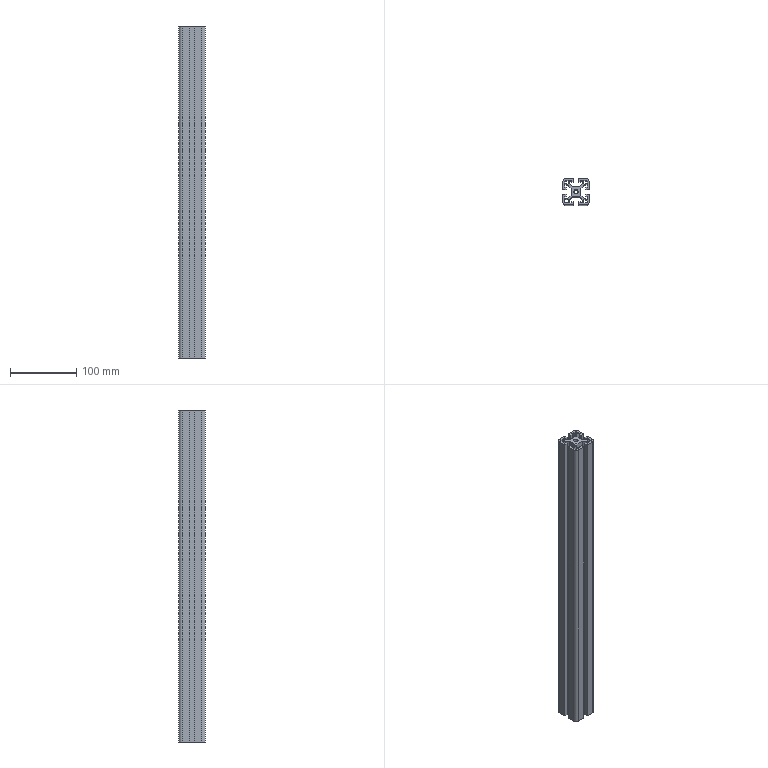Part | STEP file | 4040-500 | 1 solid | 88 faces | box 40 x 40 x 500 mm | volume 351974 mm3 | plane 78 | cylinder 10 | commonest cylinder face diameters 4 x4 10 x4 6.8 x2